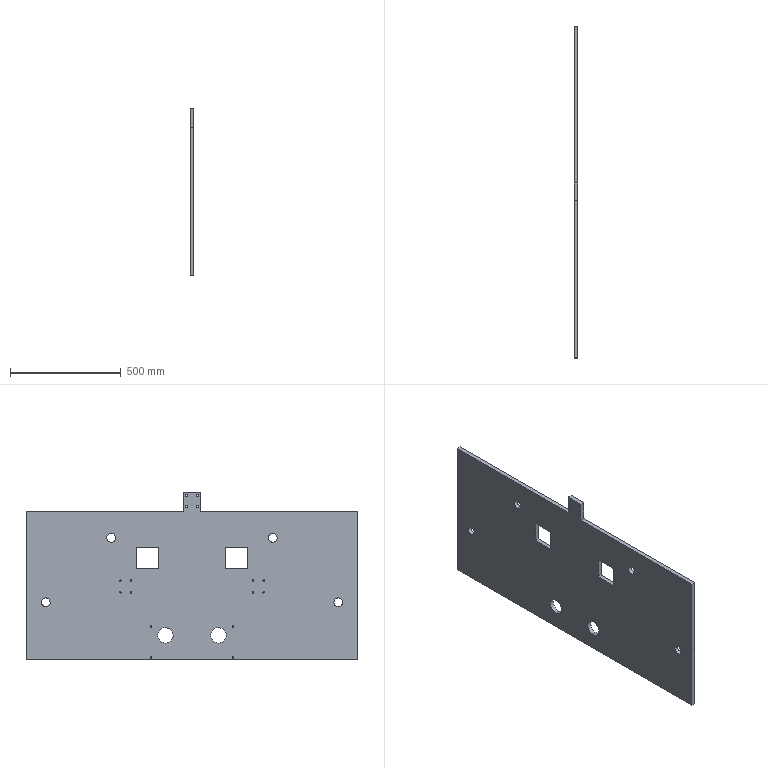Part | STEP file | Positioning_id1002_x_t | 1 solid | 62 faces | box 18 x 1500 x 757.034 mm | volume 17633619 mm3 | cylinder 44 | plane 18 | commonest cylinder face diameters 6 x24 9 x8 40 x8 70 x4